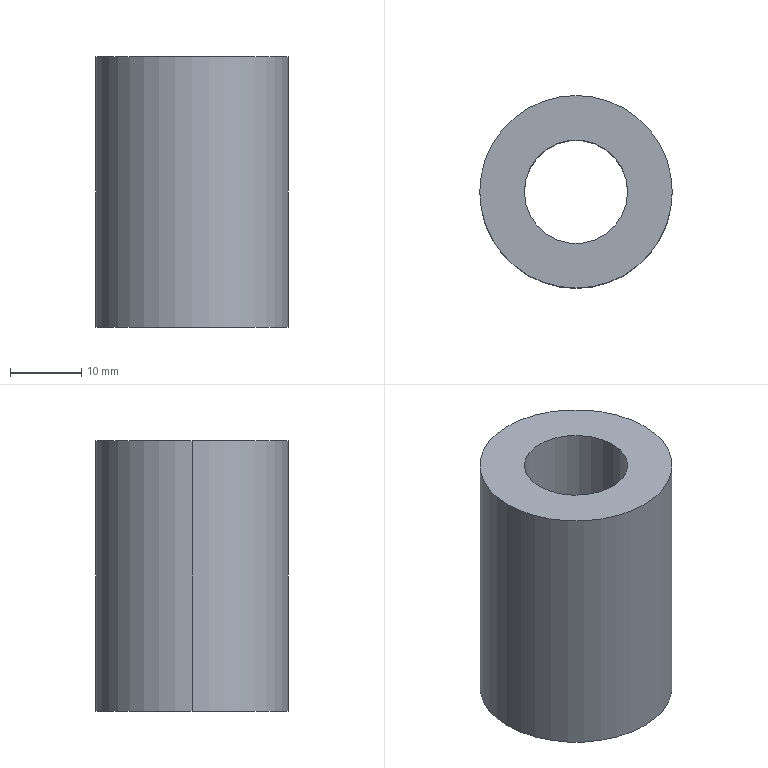Part | SolidWorks | features Extrusion 1, HoleWzd 1 | 1 solid | 6 faces | box 27 x 27 x 38 mm | volume 15482 mm3 | cylinder 4 | plane 2 | commonest cylinder face diameters 14.5 x2 27 x2
STEP:
#1=CARTESIAN_POINT('',(7.25,0.,38.));
#2=VERTEX_POINT('',#1);
#3=CARTESIAN_POINT('',(-7.25,0.,38.));
#4=VERTEX_POINT('',#3);
#5=CARTESIAN_POINT('',(0.,0.,38.));
#6=DIRECTION('',(0.,0.,-1.));
#7=DIRECTION('',(-1.,0.,0.));
#8=AXIS2_PLACEMENT_3D('',#5,#6,#7);
#9=CIRCLE('',#8,7.25);
#10=EDGE_CURVE('',#2,#4,#9,.T.);
#11=ORIENTED_EDGE('',*,*,#10,.F.);
#12=CARTESIAN_POINT('',(7.25,0.,0.));
#13=VERTEX_POINT('',#12);
#14=CARTESIAN_POINT('',(7.25,0.,0.));
#15=DIRECTION('',(0.,0.,-1.));
#16=VECTOR('',#15,1000.);
#17=LINE('',#14,#16);
#18=EDGE_CURVE('',#2,#13,#17,.T.);
#19=ORIENTED_EDGE('',*,*,#18,.T.);
#20=CARTESIAN_POINT('',(-7.25,0.,0.));
#21=VERTEX_POINT('',#20);
#22=CARTESIAN_POINT('',(0.,0.,0.));
#23=DIRECTION('',(0.,0.,-1.));
#24=DIRECTION('',(-1.,0.,0.));
#25=AXIS2_PLACEMENT_3D('',#22,#23,#24);
#26=CIRCLE('',#25,7.25);
#27=EDGE_CURVE('',#13,#21,#26,.T.);
#28=ORIENTED_EDGE('',*,*,#27,.T.);
#29=CARTESIAN_POINT('',(-7.25,0.,0.));
#30=DIRECTION('',(0.,0.,-1.));
#31=VECTOR('',#30,1000.);
#32=LINE('',#29,#31);
#33=EDGE_CURVE('',#4,#21,#32,.T.);
#34=ORIENTED_EDGE('',*,*,#33,.F.);
#35=EDGE_LOOP('',(#11,#19,#28,#34));
#36=FACE_OUTER_BOUND('',#35,.T.);
#37=CARTESIAN_POINT('',(0.,0.,0.));
#38=DIRECTION('',(0.,0.,-1.));
#39=DIRECTION('',(-1.,0.,0.));
#40=AXIS2_PLACEMENT_3D('',#37,#38,#39);
#41=CYLINDRICAL_SURFACE('',#40,7.25);
#42=ADVANCED_FACE('',(#36),#41,.F.);
#43=CARTESIAN_POINT('',(13.5,0.,38.));
#44=VERTEX_POINT('',#43);
#45=CARTESIAN_POINT('',(-13.5,0.,38.));
#46=VERTEX_POINT('',#45);
#47=CARTESIAN_POINT('',(0.,0.,38.));
#48=DIRECTION('',(0.,0.,1.));
#49=DIRECTION('',(1.,0.,0.));
#50=AXIS2_PLACEMENT_3D('',#47,#48,#49);
#51=CIRCLE('',#50,13.5);
#52=EDGE_CURVE('',#44,#46,#51,.T.);
#53=ORIENTED_EDGE('',*,*,#52,.F.);
#54=CARTESIAN_POINT('',(13.5,0.,0.));
#55=VERTEX_POINT('',#54);
#56=CARTESIAN_POINT('',(13.5,0.,38.));
#57=DIRECTION('',(0.,0.,-1.));
#58=VECTOR('',#57,1000.);
#59=LINE('',#56,#58);
#60=EDGE_CURVE('',#44,#55,#59,.T.);
#61=ORIENTED_EDGE('',*,*,#60,.T.);
#62=CARTESIAN_POINT('',(-13.5,0.,0.));
#63=VERTEX_POINT('',#62);
#64=CARTESIAN_POINT('',(0.,0.,0.));
#65=DIRECTION('',(0.,0.,1.));
#66=DIRECTION('',(1.,0.,0.));
#67=AXIS2_PLACEMENT_3D('',#64,#65,#66);
#68=CIRCLE('',#67,13.5);
#69=EDGE_CURVE('',#55,#63,#68,.T.);
#70=ORIENTED_EDGE('',*,*,#69,.T.);
#71=CARTESIAN_POINT('',(-13.5,0.,38.));
#72=DIRECTION('',(0.,0.,-1.));
#73=VECTOR('',#72,1000.);
#74=LINE('',#71,#73);
#75=EDGE_CURVE('',#46,#63,#74,.T.);
#76=ORIENTED_EDGE('',*,*,#75,.F.);
#77=EDGE_LOOP('',(#53,#61,#70,#76));
#78=FACE_OUTER_BOUND('',#77,.T.);
#79=CARTESIAN_POINT('',(0.,0.,38.));
#80=DIRECTION('',(0.,0.,-1.));
#81=DIRECTION('',(-1.,0.,0.));
#82=AXIS2_PLACEMENT_3D('',#79,#80,#81);
#83=CYLINDRICAL_SURFACE('',#82,13.5);
#84=ADVANCED_FACE('',(#78),#83,.T.);
#85=CARTESIAN_POINT('',(0.,0.,38.));
#86=DIRECTION('',(0.,0.,-1.));
#87=DIRECTION('',(-1.,0.,0.));
#88=AXIS2_PLACEMENT_3D('',#85,#86,#87);
#89=CIRCLE('',#88,7.25);
#90=EDGE_CURVE('',#4,#2,#89,.T.);
#91=ORIENTED_EDGE('',*,*,#90,.T.);
#92=ORIENTED_EDGE('',*,*,#10,.T.);
#93=EDGE_LOOP('',(#91,#92));
#94=FACE_BOUND('',#93,.T.);
#95=CARTESIAN_POINT('',(0.,0.,38.));
#96=DIRECTION('',(0.,0.,1.));
#97=DIRECTION('',(1.,0.,0.));
#98=AXIS2_PLACEMENT_3D('',#95,#96,#97);
#99=CIRCLE('',#98,13.5);
#100=EDGE_CURVE('',#46,#44,#99,.T.);
#101=ORIENTED_EDGE('',*,*,#100,.T.);
#102=ORIENTED_EDGE('',*,*,#52,.T.);
#103=EDGE_LOOP('',(#101,#102));
#104=FACE_OUTER_BOUND('',#103,.T.);
#105=CARTESIAN_POINT('',(0.,0.,38.));
#106=DIRECTION('',(0.,0.,1.));
#107=DIRECTION('',(1.,0.,0.));
#108=AXIS2_PLACEMENT_3D('',#105,#106,#107);
#109=PLANE('',#108);
#110=ADVANCED_FACE('',(#94,#104),#109,.T.);
#111=CARTESIAN_POINT('',(0.,0.,0.));
#112=DIRECTION('',(0.,0.,-1.));
#113=DIRECTION('',(-1.,0.,0.));
#114=AXIS2_PLACEMENT_3D('',#111,#112,#113);
#115=CIRCLE('',#114,7.25);
#116=EDGE_CURVE('',#21,#13,#115,.T.);
#117=ORIENTED_EDGE('',*,*,#116,.F.);
#118=ORIENTED_EDGE('',*,*,#27,.F.);
#119=EDGE_LOOP('',(#117,#118));
#120=FACE_BOUND('',#119,.T.);
#121=CARTESIAN_POINT('',(0.,0.,0.));
#122=DIRECTION('',(0.,0.,1.));
#123=DIRECTION('',(1.,0.,0.));
#124=AXIS2_PLACEMENT_3D('',#121,#122,#123);
#125=CIRCLE('',#124,13.5);
#126=EDGE_CURVE('',#63,#55,#125,.T.);
#127=ORIENTED_EDGE('',*,*,#126,.F.);
#128=ORIENTED_EDGE('',*,*,#69,.F.);
#129=EDGE_LOOP('',(#127,#128));
#130=FACE_OUTER_BOUND('',#129,.T.);
#131=CARTESIAN_POINT('',(0.,0.,0.));
#132=DIRECTION('',(0.,0.,1.));
#133=DIRECTION('',(1.,0.,0.));
#134=AXIS2_PLACEMENT_3D('',#131,#132,#133);
#135=PLANE('',#134);
#136=ADVANCED_FACE('',(#120,#130),#135,.F.);
#137=ORIENTED_EDGE('',*,*,#60,.F.);
#138=ORIENTED_EDGE('',*,*,#100,.F.);
#139=ORIENTED_EDGE('',*,*,#75,.T.);
#140=ORIENTED_EDGE('',*,*,#126,.T.);
#141=EDGE_LOOP('',(#137,#138,#139,#140));
#142=FACE_OUTER_BOUND('',#141,.T.);
#143=CARTESIAN_POINT('',(0.,0.,38.));
#144=DIRECTION('',(0.,0.,-1.));
#145=DIRECTION('',(-1.,0.,0.));
#146=AXIS2_PLACEMENT_3D('',#143,#144,#145);
#147=CYLINDRICAL_SURFACE('',#146,13.5);
#148=ADVANCED_FACE('',(#142),#147,.T.);
#149=ORIENTED_EDGE('',*,*,#18,.F.);
#150=ORIENTED_EDGE('',*,*,#90,.F.);
#151=ORIENTED_EDGE('',*,*,#33,.T.);
#152=ORIENTED_EDGE('',*,*,#116,.T.);
#153=EDGE_LOOP('',(#149,#150,#151,#152));
#154=FACE_OUTER_BOUND('',#153,.T.);
#155=CARTESIAN_POINT('',(0.,0.,0.));
#156=DIRECTION('',(0.,0.,-1.));
#157=DIRECTION('',(-1.,0.,0.));
#158=AXIS2_PLACEMENT_3D('',#155,#156,#157);
#159=CYLINDRICAL_SURFACE('',#158,7.25);
#160=ADVANCED_FACE('',(#154),#159,.F.);
#161=CLOSED_SHELL('',(#42,#84,#110,#136,#148,#160));
#162=MANIFOLD_SOLID_BREP('',#161);
#163=CARTESIAN_POINT('',(0.,0.,0.));
#164=DIRECTION('',(0.,0.,1.));
#165=DIRECTION('',(1.,0.,0.));
#166=AXIS2_PLACEMENT_3D('',#163,#164,#165);
#167=(LENGTH_UNIT()NAMED_UNIT(*)SI_UNIT(.MILLI.,.METRE.));
#168=UNCERTAINTY_MEASURE_WITH_UNIT(LENGTH_MEASURE(0.00001),#167,'','');
#169=(NAMED_UNIT(*)PLANE_ANGLE_UNIT()SI_UNIT($,.RADIAN.));
#170=(NAMED_UNIT(*)SI_UNIT($,.STERADIAN.)SOLID_ANGLE_UNIT());
#171=(GEOMETRIC_REPRESENTATION_CONTEXT(3)GLOBAL_UNCERTAINTY_ASSIGNED_CONTEXT((#168))GLOBAL_UNIT_ASSIGNED_CONTEXT((#167,#169,#170))REPRESENTATION_CONTEXT('',''));
#172=ADVANCED_BREP_SHAPE_REPRESENTATION('',(#162,#166),#171);